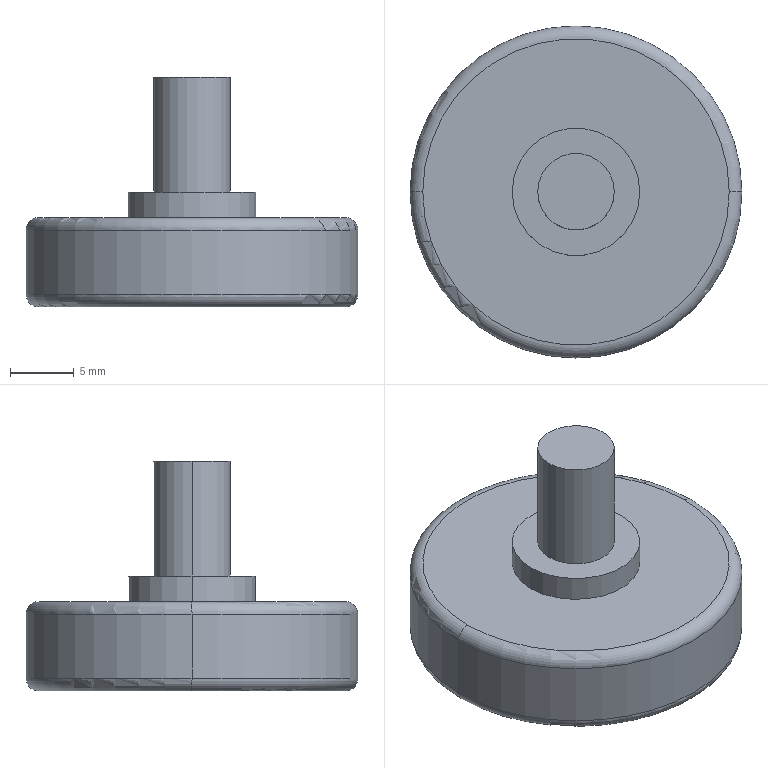Part | STEP file | Nylon roller | 1 solid | 14 faces | box 26 x 26 x 18 mm | volume 4094 mm3 | cylinder 6 | torus 4 | plane 4 | commonest cylinder face diameters 6 x2 10 x2 26 x2
STEP:
#1=CARTESIAN_POINT('',(0.,0.,0.));
#2=DIRECTION('',(0.,0.,1.));
#3=DIRECTION('',(1.,0.,0.));
#4=AXIS2_PLACEMENT_3D('',#1,#2,#3);
#5=CARTESIAN_POINT('',(3.,0.,18.));
#6=VERTEX_POINT('',#5);
#7=CARTESIAN_POINT('',(-3.,0.,18.));
#8=VERTEX_POINT('',#7);
#9=CARTESIAN_POINT('',(0.,0.,18.));
#10=DIRECTION('',(0.,0.,1.));
#11=DIRECTION('',(1.,0.,0.));
#12=AXIS2_PLACEMENT_3D('',#9,#10,#11);
#13=CIRCLE('',#12,3.);
#14=CARTESIAN_POINT('',(0.,0.,18.));
#15=DIRECTION('',(0.,0.,-1.));
#16=DIRECTION('',(-1.,0.,0.));
#17=AXIS2_PLACEMENT_3D('',#14,#15,#16);
#18=CYLINDRICAL_SURFACE('',#17,3.);
#19=CARTESIAN_POINT('',(3.142,0.));
#20=DIRECTION('',(-1.,0.));
#21=VECTOR('',#20,1.);
#22=LINE('',#19,#21);
#23=(GEOMETRIC_REPRESENTATION_CONTEXT(2)PARAMETRIC_REPRESENTATION_CONTEXT()REPRESENTATION_CONTEXT('',''));
#24=DEFINITIONAL_REPRESENTATION('',(#22),#23);
#25=PCURVE('',#18,#24);
#26=CARTESIAN_POINT('',(0.,0.,18.));
#27=DIRECTION('',(0.,0.,1.));
#28=DIRECTION('',(1.,0.,0.));
#29=AXIS2_PLACEMENT_3D('',#26,#27,#28);
#30=PLANE('',#29);
#31=CARTESIAN_POINT('',(0.,0.));
#32=DIRECTION('',(1.,0.));
#33=AXIS2_PLACEMENT_2D('',#31,#32);
#34=CIRCLE('',#33,3.);
#35=(GEOMETRIC_REPRESENTATION_CONTEXT(2)PARAMETRIC_REPRESENTATION_CONTEXT()REPRESENTATION_CONTEXT('',''));
#36=DEFINITIONAL_REPRESENTATION('',(#34),#35);
#37=PCURVE('',#30,#36);
#38=SURFACE_CURVE('',#13,(#25,#37),.PCURVE_S1.);
#39=EDGE_CURVE('',#6,#8,#38,.T.);
#40=ORIENTED_EDGE('',*,*,#39,.F.);
#41=CARTESIAN_POINT('',(3.,0.,9.));
#42=VERTEX_POINT('',#41);
#43=CARTESIAN_POINT('',(3.,0.,18.));
#44=DIRECTION('',(0.,0.,-1.));
#45=VECTOR('',#44,1.);
#46=LINE('',#43,#45);
#47=CARTESIAN_POINT('',(3.142,0.));
#48=DIRECTION('',(0.,1.));
#49=VECTOR('',#48,1.);
#50=LINE('',#47,#49);
#51=(GEOMETRIC_REPRESENTATION_CONTEXT(2)PARAMETRIC_REPRESENTATION_CONTEXT()REPRESENTATION_CONTEXT('',''));
#52=DEFINITIONAL_REPRESENTATION('',(#50),#51);
#53=PCURVE('',#18,#52);
#54=CARTESIAN_POINT('',(0.,0.,18.));
#55=DIRECTION('',(0.,0.,-1.));
#56=DIRECTION('',(-1.,0.,0.));
#57=AXIS2_PLACEMENT_3D('',#54,#55,#56);
#58=CYLINDRICAL_SURFACE('',#57,3.);
#59=CARTESIAN_POINT('',(3.142,0.));
#60=DIRECTION('',(0.,1.));
#61=VECTOR('',#60,1.);
#62=LINE('',#59,#61);
#63=(GEOMETRIC_REPRESENTATION_CONTEXT(2)PARAMETRIC_REPRESENTATION_CONTEXT()REPRESENTATION_CONTEXT('',''));
#64=DEFINITIONAL_REPRESENTATION('',(#62),#63);
#65=PCURVE('',#58,#64);
#66=SURFACE_CURVE('',#46,(#53,#65),.PCURVE_S1.);
#67=EDGE_CURVE('',#6,#42,#66,.T.);
#68=ORIENTED_EDGE('',*,*,#67,.T.);
#69=CARTESIAN_POINT('',(-3.,0.,9.));
#70=VERTEX_POINT('',#69);
#71=CARTESIAN_POINT('',(0.,0.,9.));
#72=DIRECTION('',(0.,0.,1.));
#73=DIRECTION('',(1.,0.,0.));
#74=AXIS2_PLACEMENT_3D('',#71,#72,#73);
#75=CIRCLE('',#74,3.);
#76=CARTESIAN_POINT('',(3.142,9.));
#77=DIRECTION('',(-1.,0.));
#78=VECTOR('',#77,1.);
#79=LINE('',#76,#78);
#80=(GEOMETRIC_REPRESENTATION_CONTEXT(2)PARAMETRIC_REPRESENTATION_CONTEXT()REPRESENTATION_CONTEXT('',''));
#81=DEFINITIONAL_REPRESENTATION('',(#79),#80);
#82=PCURVE('',#18,#81);
#83=CARTESIAN_POINT('',(0.,0.,9.));
#84=DIRECTION('',(0.,0.,1.));
#85=DIRECTION('',(1.,0.,0.));
#86=AXIS2_PLACEMENT_3D('',#83,#84,#85);
#87=PLANE('',#86);
#88=CARTESIAN_POINT('',(0.,0.));
#89=DIRECTION('',(1.,0.));
#90=AXIS2_PLACEMENT_2D('',#88,#89);
#91=CIRCLE('',#90,3.);
#92=(GEOMETRIC_REPRESENTATION_CONTEXT(2)PARAMETRIC_REPRESENTATION_CONTEXT()REPRESENTATION_CONTEXT('',''));
#93=DEFINITIONAL_REPRESENTATION('',(#91),#92);
#94=PCURVE('',#87,#93);
#95=SURFACE_CURVE('',#75,(#82,#94),.PCURVE_S1.);
#96=EDGE_CURVE('',#42,#70,#95,.T.);
#97=ORIENTED_EDGE('',*,*,#96,.T.);
#98=CARTESIAN_POINT('',(-3.,0.,18.));
#99=DIRECTION('',(0.,0.,-1.));
#100=VECTOR('',#99,1.);
#101=LINE('',#98,#100);
#102=CARTESIAN_POINT('',(0.,0.));
#103=DIRECTION('',(0.,1.));
#104=VECTOR('',#103,1.);
#105=LINE('',#102,#104);
#106=(GEOMETRIC_REPRESENTATION_CONTEXT(2)PARAMETRIC_REPRESENTATION_CONTEXT()REPRESENTATION_CONTEXT('',''));
#107=DEFINITIONAL_REPRESENTATION('',(#105),#106);
#108=PCURVE('',#18,#107);
#109=CARTESIAN_POINT('',(6.283,0.));
#110=DIRECTION('',(0.,1.));
#111=VECTOR('',#110,1.);
#112=LINE('',#109,#111);
#113=(GEOMETRIC_REPRESENTATION_CONTEXT(2)PARAMETRIC_REPRESENTATION_CONTEXT()REPRESENTATION_CONTEXT('',''));
#114=DEFINITIONAL_REPRESENTATION('',(#112),#113);
#115=PCURVE('',#58,#114);
#116=SURFACE_CURVE('',#101,(#108,#115),.PCURVE_S1.);
#117=EDGE_CURVE('',#8,#70,#116,.T.);
#118=ORIENTED_EDGE('',*,*,#117,.F.);
#119=EDGE_LOOP('',(#40,#68,#97,#118));
#120=FACE_BOUND('',#119,.T.);
#121=ADVANCED_FACE('',(#120),#18,.T.);
#122=CARTESIAN_POINT('',(5.,0.,9.));
#123=VERTEX_POINT('',#122);
#124=CARTESIAN_POINT('',(-5.,0.,9.));
#125=VERTEX_POINT('',#124);
#126=CARTESIAN_POINT('',(0.,0.,9.));
#127=DIRECTION('',(0.,0.,1.));
#128=DIRECTION('',(1.,0.,0.));
#129=AXIS2_PLACEMENT_3D('',#126,#127,#128);
#130=CIRCLE('',#129,5.);
#131=CARTESIAN_POINT('',(0.,0.,9.));
#132=DIRECTION('',(0.,0.,-1.));
#133=DIRECTION('',(-1.,0.,0.));
#134=AXIS2_PLACEMENT_3D('',#131,#132,#133);
#135=CYLINDRICAL_SURFACE('',#134,5.);
#136=CARTESIAN_POINT('',(3.142,0.));
#137=DIRECTION('',(-1.,0.));
#138=VECTOR('',#137,1.);
#139=LINE('',#136,#138);
#140=(GEOMETRIC_REPRESENTATION_CONTEXT(2)PARAMETRIC_REPRESENTATION_CONTEXT()REPRESENTATION_CONTEXT('',''));
#141=DEFINITIONAL_REPRESENTATION('',(#139),#140);
#142=PCURVE('',#135,#141);
#143=CARTESIAN_POINT('',(0.,0.));
#144=DIRECTION('',(1.,0.));
#145=AXIS2_PLACEMENT_2D('',#143,#144);
#146=CIRCLE('',#145,5.);
#147=(GEOMETRIC_REPRESENTATION_CONTEXT(2)PARAMETRIC_REPRESENTATION_CONTEXT()REPRESENTATION_CONTEXT('',''));
#148=DEFINITIONAL_REPRESENTATION('',(#146),#147);
#149=PCURVE('',#87,#148);
#150=SURFACE_CURVE('',#130,(#142,#149),.PCURVE_S1.);
#151=EDGE_CURVE('',#123,#125,#150,.T.);
#152=ORIENTED_EDGE('',*,*,#151,.F.);
#153=CARTESIAN_POINT('',(5.,0.,7.));
#154=VERTEX_POINT('',#153);
#155=CARTESIAN_POINT('',(5.,0.,9.));
#156=DIRECTION('',(0.,0.,-1.));
#157=VECTOR('',#156,1.);
#158=LINE('',#155,#157);
#159=CARTESIAN_POINT('',(3.142,0.));
#160=DIRECTION('',(0.,1.));
#161=VECTOR('',#160,1.);
#162=LINE('',#159,#161);
#163=(GEOMETRIC_REPRESENTATION_CONTEXT(2)PARAMETRIC_REPRESENTATION_CONTEXT()REPRESENTATION_CONTEXT('',''));
#164=DEFINITIONAL_REPRESENTATION('',(#162),#163);
#165=PCURVE('',#135,#164);
#166=CARTESIAN_POINT('',(0.,0.,9.));
#167=DIRECTION('',(0.,0.,-1.));
#168=DIRECTION('',(-1.,0.,0.));
#169=AXIS2_PLACEMENT_3D('',#166,#167,#168);
#170=CYLINDRICAL_SURFACE('',#169,5.);
#171=CARTESIAN_POINT('',(3.142,0.));
#172=DIRECTION('',(0.,1.));
#173=VECTOR('',#172,1.);
#174=LINE('',#171,#173);
#175=(GEOMETRIC_REPRESENTATION_CONTEXT(2)PARAMETRIC_REPRESENTATION_CONTEXT()REPRESENTATION_CONTEXT('',''));
#176=DEFINITIONAL_REPRESENTATION('',(#174),#175);
#177=PCURVE('',#170,#176);
#178=SURFACE_CURVE('',#158,(#165,#177),.PCURVE_S1.);
#179=EDGE_CURVE('',#123,#154,#178,.T.);
#180=ORIENTED_EDGE('',*,*,#179,.T.);
#181=CARTESIAN_POINT('',(-5.,0.,7.));
#182=VERTEX_POINT('',#181);
#183=CARTESIAN_POINT('',(0.,0.,7.));
#184=DIRECTION('',(0.,0.,1.));
#185=DIRECTION('',(1.,0.,0.));
#186=AXIS2_PLACEMENT_3D('',#183,#184,#185);
#187=CIRCLE('',#186,5.);
#188=CARTESIAN_POINT('',(3.142,2.));
#189=DIRECTION('',(-1.,0.));
#190=VECTOR('',#189,1.);
#191=LINE('',#188,#190);
#192=(GEOMETRIC_REPRESENTATION_CONTEXT(2)PARAMETRIC_REPRESENTATION_CONTEXT()REPRESENTATION_CONTEXT('',''));
#193=DEFINITIONAL_REPRESENTATION('',(#191),#192);
#194=PCURVE('',#135,#193);
#195=CARTESIAN_POINT('',(0.,0.,7.));
#196=DIRECTION('',(0.,0.,1.));
#197=DIRECTION('',(1.,0.,0.));
#198=AXIS2_PLACEMENT_3D('',#195,#196,#197);
#199=PLANE('',#198);
#200=CARTESIAN_POINT('',(0.,0.));
#201=DIRECTION('',(1.,0.));
#202=AXIS2_PLACEMENT_2D('',#200,#201);
#203=CIRCLE('',#202,5.);
#204=(GEOMETRIC_REPRESENTATION_CONTEXT(2)PARAMETRIC_REPRESENTATION_CONTEXT()REPRESENTATION_CONTEXT('',''));
#205=DEFINITIONAL_REPRESENTATION('',(#203),#204);
#206=PCURVE('',#199,#205);
#207=SURFACE_CURVE('',#187,(#194,#206),.PCURVE_S1.);
#208=EDGE_CURVE('',#154,#182,#207,.T.);
#209=ORIENTED_EDGE('',*,*,#208,.T.);
#210=CARTESIAN_POINT('',(-5.,0.,9.));
#211=DIRECTION('',(0.,0.,-1.));
#212=VECTOR('',#211,1.);
#213=LINE('',#210,#212);
#214=CARTESIAN_POINT('',(0.,0.));
#215=DIRECTION('',(0.,1.));
#216=VECTOR('',#215,1.);
#217=LINE('',#214,#216);
#218=(GEOMETRIC_REPRESENTATION_CONTEXT(2)PARAMETRIC_REPRESENTATION_CONTEXT()REPRESENTATION_CONTEXT('',''));
#219=DEFINITIONAL_REPRESENTATION('',(#217),#218);
#220=PCURVE('',#135,#219);
#221=CARTESIAN_POINT('',(6.283,0.));
#222=DIRECTION('',(0.,1.));
#223=VECTOR('',#222,1.);
#224=LINE('',#221,#223);
#225=(GEOMETRIC_REPRESENTATION_CONTEXT(2)PARAMETRIC_REPRESENTATION_CONTEXT()REPRESENTATION_CONTEXT('',''));
#226=DEFINITIONAL_REPRESENTATION('',(#224),#225);
#227=PCURVE('',#170,#226);
#228=SURFACE_CURVE('',#213,(#220,#227),.PCURVE_S1.);
#229=EDGE_CURVE('',#125,#182,#228,.T.);
#230=ORIENTED_EDGE('',*,*,#229,.F.);
#231=EDGE_LOOP('',(#152,#180,#209,#230));
#232=FACE_BOUND('',#231,.T.);
#233=ADVANCED_FACE('',(#232),#135,.T.);
#234=CARTESIAN_POINT('',(-13.,0.,6.));
#235=VERTEX_POINT('',#234);
#236=CARTESIAN_POINT('',(13.,0.,6.));
#237=VERTEX_POINT('',#236);
#238=CARTESIAN_POINT('',(0.,0.,6.));
#239=DIRECTION('',(0.,0.,-1.));
#240=DIRECTION('',(1.,0.,0.));
#241=AXIS2_PLACEMENT_3D('',#238,#239,#240);
#242=CIRCLE('',#241,13.);
#243=CARTESIAN_POINT('',(0.,0.,6.));
#244=DIRECTION('',(0.,0.,1.));
#245=DIRECTION('',(1.,0.,0.));
#246=AXIS2_PLACEMENT_3D('',#243,#244,#245);
#247=TOROIDAL_SURFACE('',#246,12.,1.);
#248=CARTESIAN_POINT('',(6.283,0.));
#249=DIRECTION('',(-1.,0.));
#250=VECTOR('',#249,1.);
#251=LINE('',#248,#250);
#252=(GEOMETRIC_REPRESENTATION_CONTEXT(2)PARAMETRIC_REPRESENTATION_CONTEXT()REPRESENTATION_CONTEXT('',''));
#253=DEFINITIONAL_REPRESENTATION('',(#251),#252);
#254=PCURVE('',#247,#253);
#255=CARTESIAN_POINT('',(0.,0.,7.));
#256=DIRECTION('',(0.,0.,-1.));
#257=DIRECTION('',(-1.,0.,0.));
#258=AXIS2_PLACEMENT_3D('',#255,#256,#257);
#259=CYLINDRICAL_SURFACE('',#258,13.);
#260=CARTESIAN_POINT('',(-3.142,1.));
#261=DIRECTION('',(1.,0.));
#262=VECTOR('',#261,1.);
#263=LINE('',#260,#262);
#264=(GEOMETRIC_REPRESENTATION_CONTEXT(2)PARAMETRIC_REPRESENTATION_CONTEXT()REPRESENTATION_CONTEXT('',''));
#265=DEFINITIONAL_REPRESENTATION('',(#263),#264);
#266=PCURVE('',#259,#265);
#267=SURFACE_CURVE('',#242,(#254,#266),.PCURVE_S1.);
#268=EDGE_CURVE('',#235,#237,#267,.T.);
#269=ORIENTED_EDGE('',*,*,#268,.F.);
#270=CARTESIAN_POINT('',(-12.,0.,7.));
#271=VERTEX_POINT('',#270);
#272=CARTESIAN_POINT('',(-12.,0.,6.));
#273=DIRECTION('',(0.,1.,0.));
#274=DIRECTION('',(-1.,0.,0.));
#275=AXIS2_PLACEMENT_3D('',#272,#273,#274);
#276=CIRCLE('',#275,1.);
#277=CARTESIAN_POINT('',(3.142,0.));
#278=DIRECTION('',(0.,1.));
#279=VECTOR('',#278,1.);
#280=LINE('',#277,#279);
#281=(GEOMETRIC_REPRESENTATION_CONTEXT(2)PARAMETRIC_REPRESENTATION_CONTEXT()REPRESENTATION_CONTEXT('',''));
#282=DEFINITIONAL_REPRESENTATION('',(#280),#281);
#283=PCURVE('',#247,#282);
#284=CARTESIAN_POINT('',(0.,0.,6.));
#285=DIRECTION('',(0.,0.,1.));
#286=DIRECTION('',(1.,0.,0.));
#287=AXIS2_PLACEMENT_3D('',#284,#285,#286);
#288=TOROIDAL_SURFACE('',#287,12.,1.);
#289=CARTESIAN_POINT('',(3.142,0.));
#290=DIRECTION('',(0.,1.));
#291=VECTOR('',#290,1.);
#292=LINE('',#289,#291);
#293=(GEOMETRIC_REPRESENTATION_CONTEXT(2)PARAMETRIC_REPRESENTATION_CONTEXT()REPRESENTATION_CONTEXT('',''));
#294=DEFINITIONAL_REPRESENTATION('',(#292),#293);
#295=PCURVE('',#288,#294);
#296=SURFACE_CURVE('',#276,(#283,#295),.PCURVE_S1.);
#297=EDGE_CURVE('',#235,#271,#296,.T.);
#298=ORIENTED_EDGE('',*,*,#297,.T.);
#299=CARTESIAN_POINT('',(12.,0.,7.));
#300=VERTEX_POINT('',#299);
#301=CARTESIAN_POINT('',(0.,0.,7.));
#302=DIRECTION('',(0.,0.,1.));
#303=DIRECTION('',(1.,0.,0.));
#304=AXIS2_PLACEMENT_3D('',#301,#302,#303);
#305=CIRCLE('',#304,12.);
#306=CARTESIAN_POINT('',(0.,1.571));
#307=DIRECTION('',(1.,0.));
#308=VECTOR('',#307,1.);
#309=LINE('',#306,#308);
#310=(GEOMETRIC_REPRESENTATION_CONTEXT(2)PARAMETRIC_REPRESENTATION_CONTEXT()REPRESENTATION_CONTEXT('',''));
#311=DEFINITIONAL_REPRESENTATION('',(#309),#310);
#312=PCURVE('',#247,#311);
#313=CARTESIAN_POINT('',(0.,0.));
#314=DIRECTION('',(1.,0.));
#315=AXIS2_PLACEMENT_2D('',#313,#314);
#316=CIRCLE('',#315,12.);
#317=(GEOMETRIC_REPRESENTATION_CONTEXT(2)PARAMETRIC_REPRESENTATION_CONTEXT()REPRESENTATION_CONTEXT('',''));
#318=DEFINITIONAL_REPRESENTATION('',(#316),#317);
#319=PCURVE('',#199,#318);
#320=SURFACE_CURVE('',#305,(#312,#319),.PCURVE_S1.);
#321=EDGE_CURVE('',#300,#271,#320,.T.);
#322=ORIENTED_EDGE('',*,*,#321,.F.);
#323=CARTESIAN_POINT('',(12.,0.,6.));
#324=DIRECTION('',(0.,-1.,0.));
#325=DIRECTION('',(0.,0.,-1.));
#326=AXIS2_PLACEMENT_3D('',#323,#324,#325);
#327=CIRCLE('',#326,1.);
#328=CARTESIAN_POINT('',(0.,-1.571));
#329=DIRECTION('',(0.,1.));
#330=VECTOR('',#329,1.);
#331=LINE('',#328,#330);
#332=(GEOMETRIC_REPRESENTATION_CONTEXT(2)PARAMETRIC_REPRESENTATION_CONTEXT()REPRESENTATION_CONTEXT('',''));
#333=DEFINITIONAL_REPRESENTATION('',(#331),#332);
#334=PCURVE('',#247,#333);
#335=CARTESIAN_POINT('',(6.283,-1.571));
#336=DIRECTION('',(0.,1.));
#337=VECTOR('',#336,1.);
#338=LINE('',#335,#337);
#339=(GEOMETRIC_REPRESENTATION_CONTEXT(2)PARAMETRIC_REPRESENTATION_CONTEXT()REPRESENTATION_CONTEXT('',''));
#340=DEFINITIONAL_REPRESENTATION('',(#338),#339);
#341=PCURVE('',#288,#340);
#342=SURFACE_CURVE('',#327,(#334,#341),.PCURVE_S1.);
#343=EDGE_CURVE('',#237,#300,#342,.T.);
#344=ORIENTED_EDGE('',*,*,#343,.F.);
#345=EDGE_LOOP('',(#269,#298,#322,#344));
#346=FACE_BOUND('',#345,.T.);
#347=ADVANCED_FACE('',(#346),#247,.T.);
#348=CARTESIAN_POINT('',(-12.,0.,0.));
#349=VERTEX_POINT('',#348);
#350=CARTESIAN_POINT('',(12.,0.,0.));
#351=VERTEX_POINT('',#350);
#352=CARTESIAN_POINT('',(0.,0.,0.));
#353=DIRECTION('',(0.,0.,-1.));
#354=DIRECTION('',(1.,0.,0.));
#355=AXIS2_PLACEMENT_3D('',#352,#353,#354);
#356=CIRCLE('',#355,12.);
#357=CARTESIAN_POINT('',(0.,0.,1.));
#358=DIRECTION('',(0.,0.,1.));
#359=DIRECTION('',(1.,0.,0.));
#360=AXIS2_PLACEMENT_3D('',#357,#358,#359);
#361=TOROIDAL_SURFACE('',#360,12.,1.);
#362=CARTESIAN_POINT('',(6.283,4.712));
#363=DIRECTION('',(-1.,0.));
#364=VECTOR('',#363,1.);
#365=LINE('',#362,#364);
#366=(GEOMETRIC_REPRESENTATION_CONTEXT(2)PARAMETRIC_REPRESENTATION_CONTEXT()REPRESENTATION_CONTEXT('',''));
#367=DEFINITIONAL_REPRESENTATION('',(#365),#366);
#368=PCURVE('',#361,#367);
#369=CARTESIAN_POINT('',(0.,0.,0.));
#370=DIRECTION('',(0.,0.,1.));
#371=DIRECTION('',(1.,0.,0.));
#372=AXIS2_PLACEMENT_3D('',#369,#370,#371);
#373=PLANE('',#372);
#374=CARTESIAN_POINT('',(12.,0.));
#375=CARTESIAN_POINT('',(12.,-20.785));
#376=CARTESIAN_POINT('',(-6.,-10.392));
#377=CARTESIAN_POINT('',(-24.,0.));
#378=CARTESIAN_POINT('',(-6.,10.392));
#379=CARTESIAN_POINT('',(12.,20.785));
#380=CARTESIAN_POINT('',(12.,0.));
#381=(BOUNDED_CURVE()B_SPLINE_CURVE(2,(#374,#375,#376,#377,#378,#379,#380),.UNSPECIFIED.,.T.,.F.)B_SPLINE_CURVE_WITH_KNOTS((1,2,2,2,2,1),(-2.094,0.,2.094,4.189,6.283,8.378),.UNSPECIFIED.)CURVE()GEOMETRIC_REPRESENTATION_ITEM()RATIONAL_B_SPLINE_CURVE((1.,0.5,1.,0.5,1.,0.5,1.))REPRESENTATION_ITEM(''));
#382=(GEOMETRIC_REPRESENTATION_CONTEXT(2)PARAMETRIC_REPRESENTATION_CONTEXT()REPRESENTATION_CONTEXT('',''));
#383=DEFINITIONAL_REPRESENTATION('',(#381),#382);
#384=PCURVE('',#373,#383);
#385=SURFACE_CURVE('',#356,(#368,#384),.PCURVE_S1.);
#386=EDGE_CURVE('',#349,#351,#385,.T.);
#387=ORIENTED_EDGE('',*,*,#386,.F.);
#388=CARTESIAN_POINT('',(-13.,0.,1.));
#389=VERTEX_POINT('',#388);
#390=CARTESIAN_POINT('',(-12.,0.,1.));
#391=DIRECTION('',(0.,1.,0.));
#392=DIRECTION('',(-1.,0.,0.));
#393=AXIS2_PLACEMENT_3D('',#390,#391,#392);
#394=CIRCLE('',#393,1.);
#395=CARTESIAN_POINT('',(3.142,0.));
#396=DIRECTION('',(0.,1.));
#397=VECTOR('',#396,1.);
#398=LINE('',#395,#397);
#399=(GEOMETRIC_REPRESENTATION_CONTEXT(2)PARAMETRIC_REPRESENTATION_CONTEXT()REPRESENTATION_CONTEXT('',''));
#400=DEFINITIONAL_REPRESENTATION('',(#398),#399);
#401=PCURVE('',#361,#400);
#402=CARTESIAN_POINT('',(0.,0.,1.));
#403=DIRECTION('',(0.,0.,1.));
#404=DIRECTION('',(1.,0.,0.));
#405=AXIS2_PLACEMENT_3D('',#402,#403,#404);
#406=TOROIDAL_SURFACE('',#405,12.,1.);
#407=CARTESIAN_POINT('',(3.142,0.));
#408=DIRECTION('',(0.,1.));
#409=VECTOR('',#408,1.);
#410=LINE('',#407,#409);
#411=(GEOMETRIC_REPRESENTATION_CONTEXT(2)PARAMETRIC_REPRESENTATION_CONTEXT()REPRESENTATION_CONTEXT('',''));
#412=DEFINITIONAL_REPRESENTATION('',(#410),#411);
#413=PCURVE('',#406,#412);
#414=SURFACE_CURVE('',#394,(#401,#413),.PCURVE_S1.);
#415=EDGE_CURVE('',#349,#389,#414,.T.);
#416=ORIENTED_EDGE('',*,*,#415,.T.);
#417=CARTESIAN_POINT('',(13.,0.,1.));
#418=VERTEX_POINT('',#417);
#419=CARTESIAN_POINT('',(0.,0.,1.));
#420=DIRECTION('',(0.,0.,1.));
#421=DIRECTION('',(1.,0.,0.));
#422=AXIS2_PLACEMENT_3D('',#419,#420,#421);
#423=CIRCLE('',#422,13.);
#424=CARTESIAN_POINT('',(0.,6.283));
#425=DIRECTION('',(1.,0.));
#426=VECTOR('',#425,1.);
#427=LINE('',#424,#426);
#428=(GEOMETRIC_REPRESENTATION_CONTEXT(2)PARAMETRIC_REPRESENTATION_CONTEXT()REPRESENTATION_CONTEXT('',''));
#429=DEFINITIONAL_REPRESENTATION('',(#427),#428);
#430=PCURVE('',#361,#429);
#431=CARTESIAN_POINT('',(3.142,6.));
#432=DIRECTION('',(-1.,0.));
#433=VECTOR('',#432,1.);
#434=LINE('',#431,#433);
#435=(GEOMETRIC_REPRESENTATION_CONTEXT(2)PARAMETRIC_REPRESENTATION_CONTEXT()REPRESENTATION_CONTEXT('',''));
#436=DEFINITIONAL_REPRESENTATION('',(#434),#435);
#437=PCURVE('',#259,#436);
#438=SURFACE_CURVE('',#423,(#430,#437),.PCURVE_S1.);
#439=EDGE_CURVE('',#418,#389,#438,.T.);
#440=ORIENTED_EDGE('',*,*,#439,.F.);
#441=CARTESIAN_POINT('',(12.,0.,1.));
#442=DIRECTION('',(0.,-1.,0.));
#443=DIRECTION('',(0.,0.,-1.));
#444=AXIS2_PLACEMENT_3D('',#441,#442,#443);
#445=CIRCLE('',#444,1.);
#446=CARTESIAN_POINT('',(0.,4.712));
#447=DIRECTION('',(0.,1.));
#448=VECTOR('',#447,1.);
#449=LINE('',#446,#448);
#450=(GEOMETRIC_REPRESENTATION_CONTEXT(2)PARAMETRIC_REPRESENTATION_CONTEXT()REPRESENTATION_CONTEXT('',''));
#451=DEFINITIONAL_REPRESENTATION('',(#449),#450);
#452=PCURVE('',#361,#451);
#453=CARTESIAN_POINT('',(6.283,4.712));
#454=DIRECTION('',(0.,1.));
#455=VECTOR('',#454,1.);
#456=LINE('',#453,#455);
#457=(GEOMETRIC_REPRESENTATION_CONTEXT(2)PARAMETRIC_REPRESENTATION_CONTEXT()REPRESENTATION_CONTEXT('',''));
#458=DEFINITIONAL_REPRESENTATION('',(#456),#457);
#459=PCURVE('',#406,#458);
#460=SURFACE_CURVE('',#445,(#452,#459),.PCURVE_S1.);
#461=EDGE_CURVE('',#351,#418,#460,.T.);
#462=ORIENTED_EDGE('',*,*,#461,.F.);
#463=EDGE_LOOP('',(#387,#416,#440,#462));
#464=FACE_BOUND('',#463,.T.);
#465=ADVANCED_FACE('',(#464),#361,.T.);
#466=ORIENTED_EDGE('',*,*,#268,.T.);
#467=CARTESIAN_POINT('',(13.,0.,7.));
#468=DIRECTION('',(0.,0.,-1.));
#469=VECTOR('',#468,1.);
#470=LINE('',#467,#469);
#471=CARTESIAN_POINT('',(3.142,0.));
#472=DIRECTION('',(0.,1.));
#473=VECTOR('',#472,1.);
#474=LINE('',#471,#473);
#475=(GEOMETRIC_REPRESENTATION_CONTEXT(2)PARAMETRIC_REPRESENTATION_CONTEXT()REPRESENTATION_CONTEXT('',''));
#476=DEFINITIONAL_REPRESENTATION('',(#474),#475);
#477=PCURVE('',#259,#476);
#478=CARTESIAN_POINT('',(0.,0.,7.));
#479=DIRECTION('',(0.,0.,-1.));
#480=DIRECTION('',(-1.,0.,0.));
#481=AXIS2_PLACEMENT_3D('',#478,#479,#480);
#482=CYLINDRICAL_SURFACE('',#481,13.);
#483=CARTESIAN_POINT('',(3.142,0.));
#484=DIRECTION('',(0.,1.));
#485=VECTOR('',#484,1.);
#486=LINE('',#483,#485);
#487=(GEOMETRIC_REPRESENTATION_CONTEXT(2)PARAMETRIC_REPRESENTATION_CONTEXT()REPRESENTATION_CONTEXT('',''));
#488=DEFINITIONAL_REPRESENTATION('',(#486),#487);
#489=PCURVE('',#482,#488);
#490=SURFACE_CURVE('',#470,(#477,#489),.PCURVE_S1.);
#491=EDGE_CURVE('',#237,#418,#490,.T.);
#492=ORIENTED_EDGE('',*,*,#491,.T.);
#493=ORIENTED_EDGE('',*,*,#439,.T.);
#494=CARTESIAN_POINT('',(-13.,0.,7.));
#495=DIRECTION('',(0.,0.,-1.));
#496=VECTOR('',#495,1.);
#497=LINE('',#494,#496);
#498=CARTESIAN_POINT('',(0.,0.));
#499=DIRECTION('',(0.,1.));
#500=VECTOR('',#499,1.);
#501=LINE('',#498,#500);
#502=(GEOMETRIC_REPRESENTATION_CONTEXT(2)PARAMETRIC_REPRESENTATION_CONTEXT()REPRESENTATION_CONTEXT('',''));
#503=DEFINITIONAL_REPRESENTATION('',(#501),#502);
#504=PCURVE('',#259,#503);
#505=CARTESIAN_POINT('',(6.283,0.));
#506=DIRECTION('',(0.,1.));
#507=VECTOR('',#506,1.);
#508=LINE('',#505,#507);
#509=(GEOMETRIC_REPRESENTATION_CONTEXT(2)PARAMETRIC_REPRESENTATION_CONTEXT()REPRESENTATION_CONTEXT('',''));
#510=DEFINITIONAL_REPRESENTATION('',(#508),#509);
#511=PCURVE('',#482,#510);
#512=SURFACE_CURVE('',#497,(#504,#511),.PCURVE_S1.);
#513=EDGE_CURVE('',#235,#389,#512,.T.);
#514=ORIENTED_EDGE('',*,*,#513,.F.);
#515=EDGE_LOOP('',(#466,#492,#493,#514));
#516=FACE_BOUND('',#515,.T.);
#517=ADVANCED_FACE('',(#516),#259,.T.);
#518=CARTESIAN_POINT('',(0.,0.,9.));
#519=DIRECTION('',(0.,0.,1.));
#520=DIRECTION('',(1.,0.,0.));
#521=AXIS2_PLACEMENT_3D('',#518,#519,#520);
#522=CIRCLE('',#521,5.);
#523=CARTESIAN_POINT('',(0.,0.));
#524=DIRECTION('',(1.,0.));
#525=AXIS2_PLACEMENT_2D('',#523,#524);
#526=CIRCLE('',#525,5.);
#527=(GEOMETRIC_REPRESENTATION_CONTEXT(2)PARAMETRIC_REPRESENTATION_CONTEXT()REPRESENTATION_CONTEXT('',''));
#528=DEFINITIONAL_REPRESENTATION('',(#526),#527);
#529=PCURVE('',#87,#528);
#530=CARTESIAN_POINT('',(9.425,0.));
#531=DIRECTION('',(-1.,0.));
#532=VECTOR('',#531,1.);
#533=LINE('',#530,#532);
#534=(GEOMETRIC_REPRESENTATION_CONTEXT(2)PARAMETRIC_REPRESENTATION_CONTEXT()REPRESENTATION_CONTEXT('',''));
#535=DEFINITIONAL_REPRESENTATION('',(#533),#534);
#536=PCURVE('',#170,#535);
#537=SURFACE_CURVE('',#522,(#529,#536),.PCURVE_S1.);
#538=EDGE_CURVE('',#125,#123,#537,.T.);
#539=ORIENTED_EDGE('',*,*,#538,.T.);
#540=ORIENTED_EDGE('',*,*,#151,.T.);
#541=EDGE_LOOP('',(#539,#540));
#542=FACE_BOUND('',#541,.T.);
#543=CARTESIAN_POINT('',(0.,0.,9.));
#544=DIRECTION('',(0.,0.,1.));
#545=DIRECTION('',(1.,0.,0.));
#546=AXIS2_PLACEMENT_3D('',#543,#544,#545);
#547=CIRCLE('',#546,3.);
#548=CARTESIAN_POINT('',(0.,0.));
#549=DIRECTION('',(1.,0.));
#550=AXIS2_PLACEMENT_2D('',#548,#549);
#551=CIRCLE('',#550,3.);
#552=(GEOMETRIC_REPRESENTATION_CONTEXT(2)PARAMETRIC_REPRESENTATION_CONTEXT()REPRESENTATION_CONTEXT('',''));
#553=DEFINITIONAL_REPRESENTATION('',(#551),#552);
#554=PCURVE('',#87,#553);
#555=CARTESIAN_POINT('',(9.425,9.));
#556=DIRECTION('',(-1.,0.));
#557=VECTOR('',#556,1.);
#558=LINE('',#555,#557);
#559=(GEOMETRIC_REPRESENTATION_CONTEXT(2)PARAMETRIC_REPRESENTATION_CONTEXT()REPRESENTATION_CONTEXT('',''));
#560=DEFINITIONAL_REPRESENTATION('',(#558),#559);
#561=PCURVE('',#58,#560);
#562=SURFACE_CURVE('',#547,(#554,#561),.PCURVE_S1.);
#563=EDGE_CURVE('',#70,#42,#562,.T.);
#564=ORIENTED_EDGE('',*,*,#563,.F.);
#565=ORIENTED_EDGE('',*,*,#96,.F.);
#566=EDGE_LOOP('',(#564,#565));
#567=FACE_BOUND('',#566,.T.);
#568=ADVANCED_FACE('',(#542,#567),#87,.T.);
#569=ORIENTED_EDGE('',*,*,#321,.T.);
#570=CARTESIAN_POINT('',(0.,0.,7.));
#571=DIRECTION('',(0.,0.,1.));
#572=DIRECTION('',(1.,0.,0.));
#573=AXIS2_PLACEMENT_3D('',#570,#571,#572);
#574=CIRCLE('',#573,12.);
#575=CARTESIAN_POINT('',(0.,0.));
#576=DIRECTION('',(1.,0.));
#577=AXIS2_PLACEMENT_2D('',#575,#576);
#578=CIRCLE('',#577,12.);
#579=(GEOMETRIC_REPRESENTATION_CONTEXT(2)PARAMETRIC_REPRESENTATION_CONTEXT()REPRESENTATION_CONTEXT('',''));
#580=DEFINITIONAL_REPRESENTATION('',(#578),#579);
#581=PCURVE('',#199,#580);
#582=CARTESIAN_POINT('',(0.,1.571));
#583=DIRECTION('',(1.,0.));
#584=VECTOR('',#583,1.);
#585=LINE('',#582,#584);
#586=(GEOMETRIC_REPRESENTATION_CONTEXT(2)PARAMETRIC_REPRESENTATION_CONTEXT()REPRESENTATION_CONTEXT('',''));
#587=DEFINITIONAL_REPRESENTATION('',(#585),#586);
#588=PCURVE('',#288,#587);
#589=SURFACE_CURVE('',#574,(#581,#588),.PCURVE_S1.);
#590=EDGE_CURVE('',#271,#300,#589,.T.);
#591=ORIENTED_EDGE('',*,*,#590,.T.);
#592=EDGE_LOOP('',(#569,#591));
#593=FACE_BOUND('',#592,.T.);
#594=CARTESIAN_POINT('',(0.,0.,7.));
#595=DIRECTION('',(0.,0.,1.));
#596=DIRECTION('',(1.,0.,0.));
#597=AXIS2_PLACEMENT_3D('',#594,#595,#596);
#598=CIRCLE('',#597,5.);
#599=CARTESIAN_POINT('',(0.,0.));
#600=DIRECTION('',(1.,0.));
#601=AXIS2_PLACEMENT_2D('',#599,#600);
#602=CIRCLE('',#601,5.);
#603=(GEOMETRIC_REPRESENTATION_CONTEXT(2)PARAMETRIC_REPRESENTATION_CONTEXT()REPRESENTATION_CONTEXT('',''));
#604=DEFINITIONAL_REPRESENTATION('',(#602),#603);
#605=PCURVE('',#199,#604);
#606=CARTESIAN_POINT('',(9.425,2.));
#607=DIRECTION('',(-1.,0.));
#608=VECTOR('',#607,1.);
#609=LINE('',#606,#608);
#610=(GEOMETRIC_REPRESENTATION_CONTEXT(2)PARAMETRIC_REPRESENTATION_CONTEXT()REPRESENTATION_CONTEXT('',''));
#611=DEFINITIONAL_REPRESENTATION('',(#609),#610);
#612=PCURVE('',#170,#611);
#613=SURFACE_CURVE('',#598,(#605,#612),.PCURVE_S1.);
#614=EDGE_CURVE('',#182,#154,#613,.T.);
#615=ORIENTED_EDGE('',*,*,#614,.F.);
#616=ORIENTED_EDGE('',*,*,#208,.F.);
#617=EDGE_LOOP('',(#615,#616));
#618=FACE_BOUND('',#617,.T.);
#619=ADVANCED_FACE('',(#593,#618),#199,.T.);
#620=ORIENTED_EDGE('',*,*,#491,.F.);
#621=CARTESIAN_POINT('',(0.,0.,6.));
#622=DIRECTION('',(0.,0.,-1.));
#623=DIRECTION('',(1.,0.,0.));
#624=AXIS2_PLACEMENT_3D('',#621,#622,#623);
#625=CIRCLE('',#624,13.);
#626=CARTESIAN_POINT('',(3.142,1.));
#627=DIRECTION('',(1.,0.));
#628=VECTOR('',#627,1.);
#629=LINE('',#626,#628);
#630=(GEOMETRIC_REPRESENTATION_CONTEXT(2)PARAMETRIC_REPRESENTATION_CONTEXT()REPRESENTATION_CONTEXT('',''));
#631=DEFINITIONAL_REPRESENTATION('',(#629),#630);
#632=PCURVE('',#482,#631);
#633=CARTESIAN_POINT('',(6.283,0.));
#634=DIRECTION('',(-1.,0.));
#635=VECTOR('',#634,1.);
#636=LINE('',#633,#635);
#637=(GEOMETRIC_REPRESENTATION_CONTEXT(2)PARAMETRIC_REPRESENTATION_CONTEXT()REPRESENTATION_CONTEXT('',''));
#638=DEFINITIONAL_REPRESENTATION('',(#636),#637);
#639=PCURVE('',#288,#638);
#640=SURFACE_CURVE('',#625,(#632,#639),.PCURVE_S1.);
#641=EDGE_CURVE('',#237,#235,#640,.T.);
#642=ORIENTED_EDGE('',*,*,#641,.T.);
#643=ORIENTED_EDGE('',*,*,#513,.T.);
#644=CARTESIAN_POINT('',(0.,0.,1.));
#645=DIRECTION('',(0.,0.,1.));
#646=DIRECTION('',(1.,0.,0.));
#647=AXIS2_PLACEMENT_3D('',#644,#645,#646);
#648=CIRCLE('',#647,13.);
#649=CARTESIAN_POINT('',(9.425,6.));
#650=DIRECTION('',(-1.,0.));
#651=VECTOR('',#650,1.);
#652=LINE('',#649,#651);
#653=(GEOMETRIC_REPRESENTATION_CONTEXT(2)PARAMETRIC_REPRESENTATION_CONTEXT()REPRESENTATION_CONTEXT('',''));
#654=DEFINITIONAL_REPRESENTATION('',(#652),#653);
#655=PCURVE('',#482,#654);
#656=CARTESIAN_POINT('',(0.,6.283));
#657=DIRECTION('',(1.,0.));
#658=VECTOR('',#657,1.);
#659=LINE('',#656,#658);
#660=(GEOMETRIC_REPRESENTATION_CONTEXT(2)PARAMETRIC_REPRESENTATION_CONTEXT()REPRESENTATION_CONTEXT('',''));
#661=DEFINITIONAL_REPRESENTATION('',(#659),#660);
#662=PCURVE('',#406,#661);
#663=SURFACE_CURVE('',#648,(#655,#662),.PCURVE_S1.);
#664=EDGE_CURVE('',#389,#418,#663,.T.);
#665=ORIENTED_EDGE('',*,*,#664,.T.);
#666=EDGE_LOOP('',(#620,#642,#643,#665));
#667=FACE_BOUND('',#666,.T.);
#668=ADVANCED_FACE('',(#667),#482,.T.);
#669=CARTESIAN_POINT('',(0.,0.,0.));
#670=DIRECTION('',(0.,0.,-1.));
#671=DIRECTION('',(1.,0.,0.));
#672=AXIS2_PLACEMENT_3D('',#669,#670,#671);
#673=CIRCLE('',#672,12.);
#674=CARTESIAN_POINT('',(12.,0.));
#675=CARTESIAN_POINT('',(12.,-20.785));
#676=CARTESIAN_POINT('',(-6.,-10.392));
#677=CARTESIAN_POINT('',(-24.,0.));
#678=CARTESIAN_POINT('',(-6.,10.392));
#679=CARTESIAN_POINT('',(12.,20.785));
#680=CARTESIAN_POINT('',(12.,0.));
#681=(BOUNDED_CURVE()B_SPLINE_CURVE(2,(#674,#675,#676,#677,#678,#679,#680),.UNSPECIFIED.,.T.,.F.)B_SPLINE_CURVE_WITH_KNOTS((1,2,2,2,2,1),(-2.094,0.,2.094,4.189,6.283,8.378),.UNSPECIFIED.)CURVE()GEOMETRIC_REPRESENTATION_ITEM()RATIONAL_B_SPLINE_CURVE((1.,0.5,1.,0.5,1.,0.5,1.))REPRESENTATION_ITEM(''));
#682=(GEOMETRIC_REPRESENTATION_CONTEXT(2)PARAMETRIC_REPRESENTATION_CONTEXT()REPRESENTATION_CONTEXT('',''));
#683=DEFINITIONAL_REPRESENTATION('',(#681),#682);
#684=PCURVE('',#373,#683);
#685=CARTESIAN_POINT('',(6.283,4.712));
#686=DIRECTION('',(-1.,0.));
#687=VECTOR('',#686,1.);
#688=LINE('',#685,#687);
#689=(GEOMETRIC_REPRESENTATION_CONTEXT(2)PARAMETRIC_REPRESENTATION_CONTEXT()REPRESENTATION_CONTEXT('',''));
#690=DEFINITIONAL_REPRESENTATION('',(#688),#689);
#691=PCURVE('',#406,#690);
#692=SURFACE_CURVE('',#673,(#684,#691),.PCURVE_S1.);
#693=EDGE_CURVE('',#351,#349,#692,.T.);
#694=ORIENTED_EDGE('',*,*,#693,.T.);
#695=ORIENTED_EDGE('',*,*,#386,.T.);
#696=EDGE_LOOP('',(#694,#695));
#697=FACE_BOUND('',#696,.T.);
#698=ADVANCED_FACE('',(#697),#373,.F.);
#699=ORIENTED_EDGE('',*,*,#415,.F.);
#700=ORIENTED_EDGE('',*,*,#693,.F.);
#701=ORIENTED_EDGE('',*,*,#461,.T.);
#702=ORIENTED_EDGE('',*,*,#664,.F.);
#703=EDGE_LOOP('',(#699,#700,#701,#702));
#704=FACE_BOUND('',#703,.T.);
#705=ADVANCED_FACE('',(#704),#406,.T.);
#706=ORIENTED_EDGE('',*,*,#297,.F.);
#707=ORIENTED_EDGE('',*,*,#641,.F.);
#708=ORIENTED_EDGE('',*,*,#343,.T.);
#709=ORIENTED_EDGE('',*,*,#590,.F.);
#710=EDGE_LOOP('',(#706,#707,#708,#709));
#711=FACE_BOUND('',#710,.T.);
#712=ADVANCED_FACE('',(#711),#288,.T.);
#713=ORIENTED_EDGE('',*,*,#179,.F.);
#714=ORIENTED_EDGE('',*,*,#538,.F.);
#715=ORIENTED_EDGE('',*,*,#229,.T.);
#716=ORIENTED_EDGE('',*,*,#614,.T.);
#717=EDGE_LOOP('',(#713,#714,#715,#716));
#718=FACE_BOUND('',#717,.T.);
#719=ADVANCED_FACE('',(#718),#170,.T.);
#720=ORIENTED_EDGE('',*,*,#67,.F.);
#721=CARTESIAN_POINT('',(0.,0.,18.));
#722=DIRECTION('',(0.,0.,1.));
#723=DIRECTION('',(1.,0.,0.));
#724=AXIS2_PLACEMENT_3D('',#721,#722,#723);
#725=CIRCLE('',#724,3.);
#726=CARTESIAN_POINT('',(9.425,0.));
#727=DIRECTION('',(-1.,0.));
#728=VECTOR('',#727,1.);
#729=LINE('',#726,#728);
#730=(GEOMETRIC_REPRESENTATION_CONTEXT(2)PARAMETRIC_REPRESENTATION_CONTEXT()REPRESENTATION_CONTEXT('',''));
#731=DEFINITIONAL_REPRESENTATION('',(#729),#730);
#732=PCURVE('',#58,#731);
#733=CARTESIAN_POINT('',(0.,0.));
#734=DIRECTION('',(1.,0.));
#735=AXIS2_PLACEMENT_2D('',#733,#734);
#736=CIRCLE('',#735,3.);
#737=(GEOMETRIC_REPRESENTATION_CONTEXT(2)PARAMETRIC_REPRESENTATION_CONTEXT()REPRESENTATION_CONTEXT('',''));
#738=DEFINITIONAL_REPRESENTATION('',(#736),#737);
#739=PCURVE('',#30,#738);
#740=SURFACE_CURVE('',#725,(#732,#739),.PCURVE_S1.);
#741=EDGE_CURVE('',#8,#6,#740,.T.);
#742=ORIENTED_EDGE('',*,*,#741,.F.);
#743=ORIENTED_EDGE('',*,*,#117,.T.);
#744=ORIENTED_EDGE('',*,*,#563,.T.);
#745=EDGE_LOOP('',(#720,#742,#743,#744));
#746=FACE_BOUND('',#745,.T.);
#747=ADVANCED_FACE('',(#746),#58,.T.);
#748=ORIENTED_EDGE('',*,*,#741,.T.);
#749=ORIENTED_EDGE('',*,*,#39,.T.);
#750=EDGE_LOOP('',(#748,#749));
#751=FACE_BOUND('',#750,.T.);
#752=ADVANCED_FACE('',(#751),#30,.T.);
#753=CLOSED_SHELL('',(#121,#233,#347,#465,#517,#568,#619,#668,#698,#705,#712,#719,#747,#752));
#754=MANIFOLD_SOLID_BREP('',#753);
#755=(LENGTH_UNIT()NAMED_UNIT(*)SI_UNIT(.MILLI.,.METRE.));
#756=UNCERTAINTY_MEASURE_WITH_UNIT(LENGTH_MEASURE(0.0000001),#755,'','');
#757=(NAMED_UNIT(*)PLANE_ANGLE_UNIT()SI_UNIT($,.RADIAN.));
#758=(NAMED_UNIT(*)SI_UNIT($,.STERADIAN.)SOLID_ANGLE_UNIT());
#759=(GEOMETRIC_REPRESENTATION_CONTEXT(3)GLOBAL_UNCERTAINTY_ASSIGNED_CONTEXT((#756))GLOBAL_UNIT_ASSIGNED_CONTEXT((#755,#757,#758))REPRESENTATION_CONTEXT('',''));
#760=ADVANCED_BREP_SHAPE_REPRESENTATION('',(#4,#754),#759);